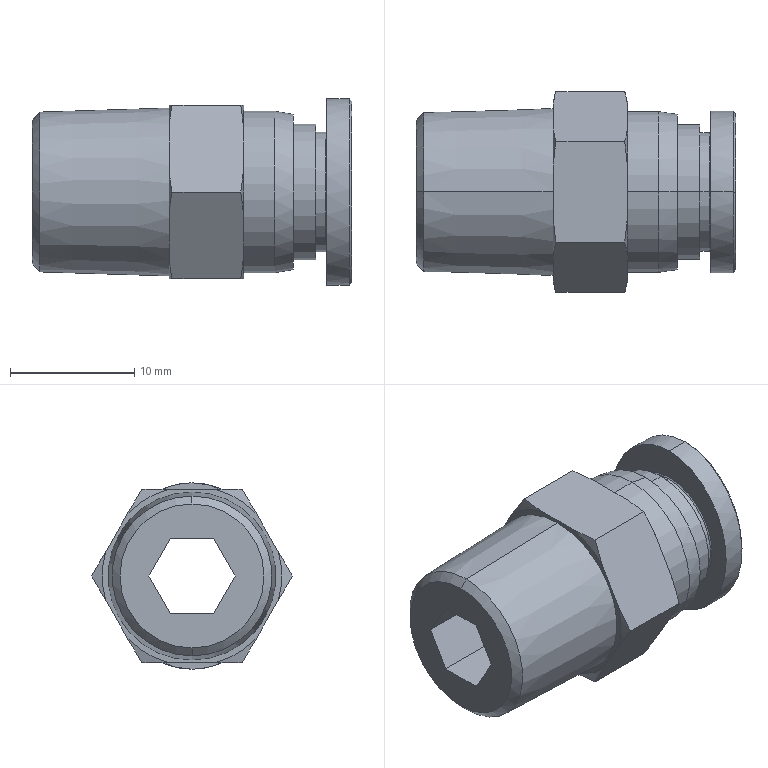Part | STEP file | upright fitting APC8-02 | 1 solid | 54 faces | box 25.7 x 16.166 x 15 mm | volume 2429 mm3 | cone 22 | plane 20 | cylinder 8 | spline 4 | commonest cylinder face diameters 8 x2 9.6 x2 10.9 x2 13 x2